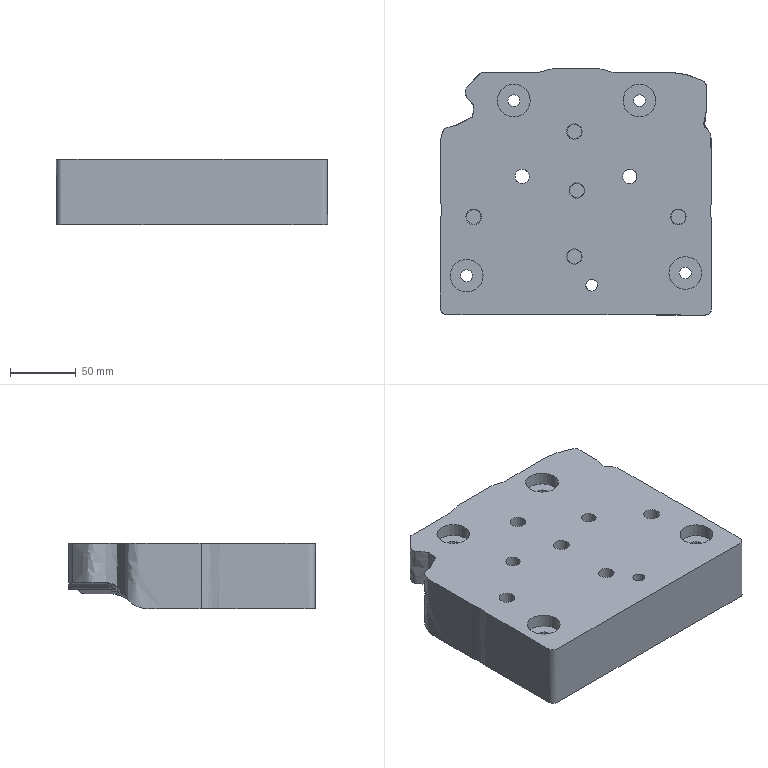Part | NX | features solid 2 | 1 solid | 110 faces | box 206.958 x 188.005 x 50.004 mm | volume 1677046 mm3 | spline 49 | cylinder 31 | plane 23 | cone 7 | commonest cylinder face diameters 12 x5 25 x5 9 x4 14 x4 11 x3 32 x3